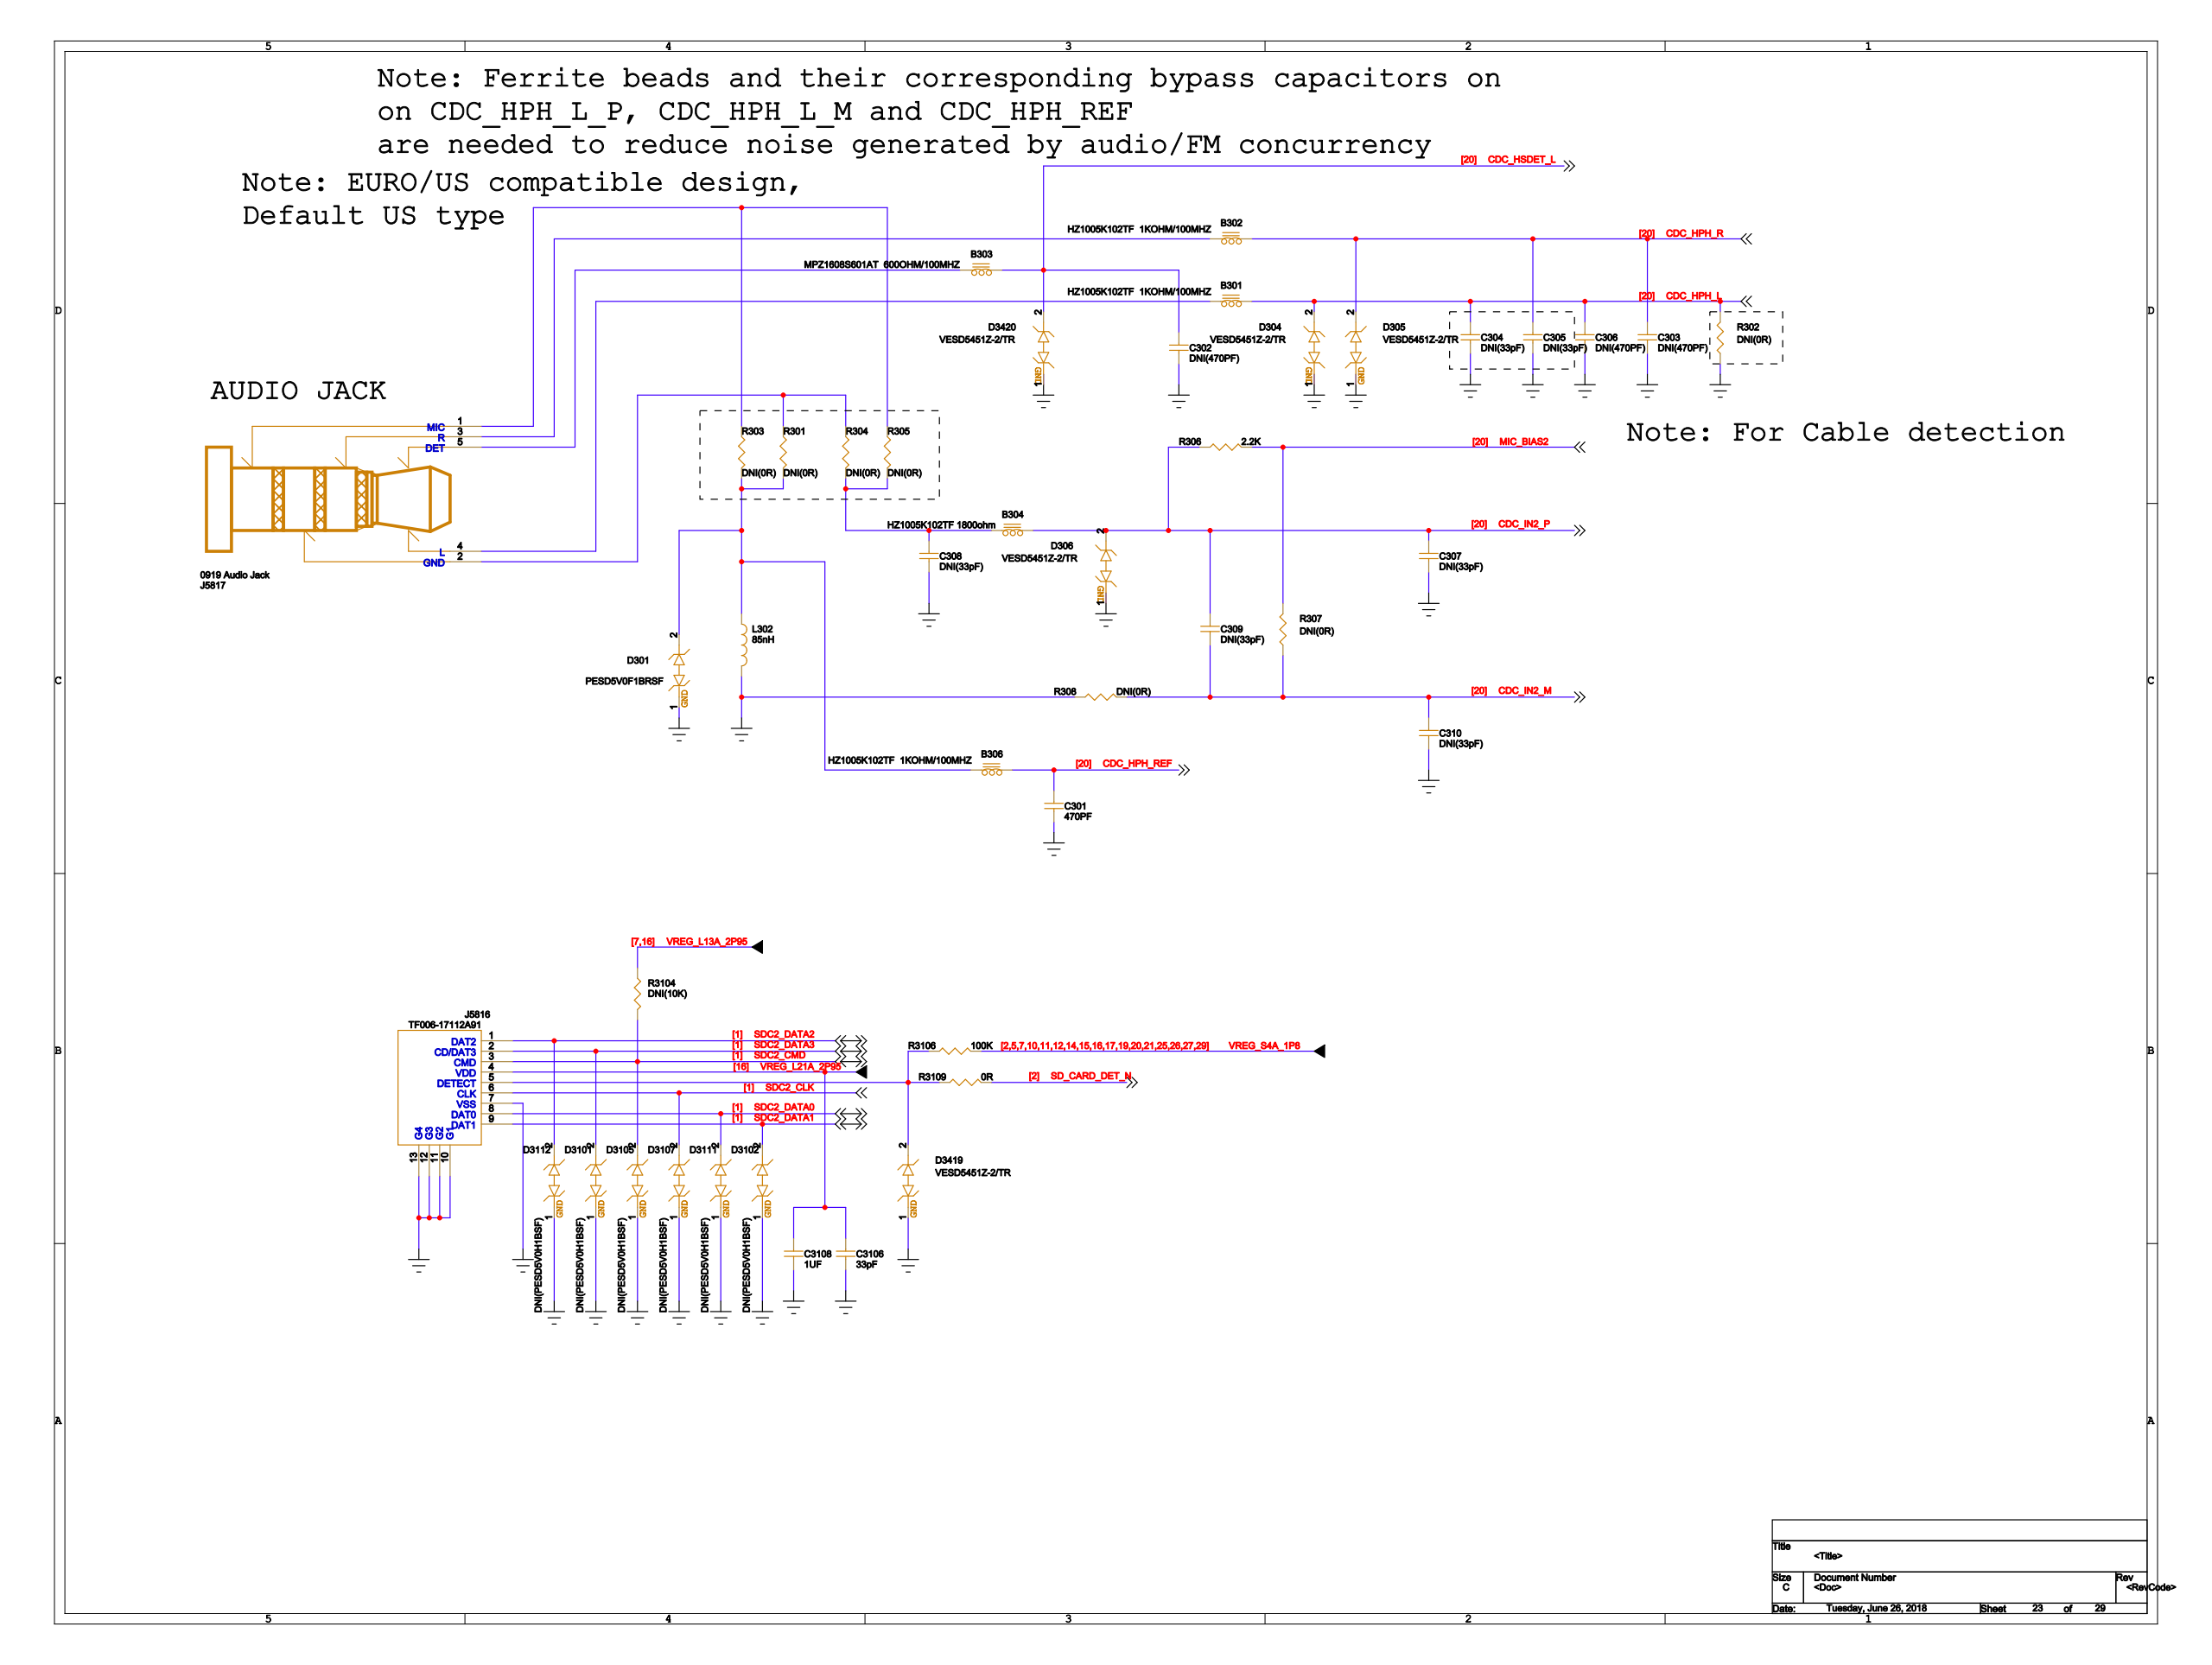Circuit board | Cadence Allegro | 802 parts | 566 nets | one sheet of the schematic
Parts on this sheet (reference | value | footprint):
B301 | HZ1005K102TF  1KOHM/100MHZ | FB0402
B302 | HZ1005K102TF  1KOHM/100MHZ | FB0402
B303 | MPZ1608S601AT  600OHM/100MHZ | FB0603_TDK
B304 | HZ1005K102TF 1800ohm | FB0402
B306 | HZ1005K102TF  1KOHM/100MHZ | FB0402
C301 | 470PF | C0201
C302 | DNI(470PF) | C0201
C303 | DNI(470PF) | C0201
C304 | DNI(33pF) | C0402
C305 | DNI(33pF) | C0402
C306 | DNI(470PF) | C0201
C307 | DNI(33pF) | C0402
C308 | DNI(33pF) | C0402
C309 | DNI(33pF) | C0402
C310 | DNI(33pF) | C0402
C3106 | 33pF | C0402
C3108 | 1uF | C0201
D301 | PESD5V0F1BRSF | DSN0603-2
D304 | VESD5451Z-2/TR | DFN0603-2L
D305 | VESD5451Z-2/TR | DFN0603-2L
D306 | VESD5451Z-2/TR | DFN0603-2L
D3419 | VESD5451Z-2/TR | DFN0603-2L
D3420 | VESD5451Z-2/TR | DFN0603-2L
J5816 | TF006-17112A91 | TF_TF006-17116A91
J5817 | 0919 Audio Jack | HP_0919_AUDIO_JACK
L302 | 85nH | L0603_LQW18CNR33J00D
R301 | DNI(0R) | R0603
R302 | DNI(0R) | R0603
R303 | DNI(0R) | R0603
R304 | DNI(0R) | R0603
R305 | DNI(0R) | R0603
R306 | 2.2K | R0201
R307 | DNI(0R) | R0603
R308 | DNI(0R) | R0603
R3104 | DNI(10K) | R0201
R3106 | 100K | R0201
R3109 | 0R | R0201
Nets of these parts (net: part-pin ...):
GND: C301-2 C302-2 C303-2 C304-2 C305-2 C306-2 C307-2 C308-2 C310-2 C3106-2 C3108-2 D301-1 D304-1 D305-1 D306-1 D3419-1 D3420-1 J5816-7 J5816-10 J5816-11 J5816-12 J5816-13 L302-2 R302-1 R308-1
SDC2_DATA3: J5816-2
SDC2_DATA1: J5816-9
SDC2_CMD: J5816-3 R3104-2
SDC2_CLK: J5816-6
SDC2_DATA0: J5816-8
SDC2_DATA2: J5816-1
VREG_S4A_1P8: R3106-2
CDC_IN2_M: C309-2 C310-1 R307-1 R308-2
CDC_IN2_P: B304-2 C307-1 C309-1 D306-2 R306-1
MIC_BIAS2: R306-2 R307-2
N373960: D3419-2 J5816-5 R3106-1 R3109-1
SD_CARD_DET_N: R3109-2
CDC_HPH_L: B301-2 C304-1 C306-1 D304-2 R302-2
CDC_HPH_R: B302-2 C303-1 C305-1 D305-2
CDC_HSDET_L: B303-2 C302-1 D3420-2
VREG_L13A_2P95: R3104-1
VREG_L21A_2P95: C3106-1 C3108-1 J5816-4
N371423: B301-1 J5817-4
N371393: B302-1 J5817-3
N369670: B306-1 D301-2 L302-1 R301-2 R303-2
CDC_HPH_REF: B306-2 C301-1
N371408: B303-1 J5817-5
N369733: B304-1 C308-1 R304-2 R305-2
N369687: J5817-2 R301-1 R304-1
N369604: J5817-1 R303-1 R305-1